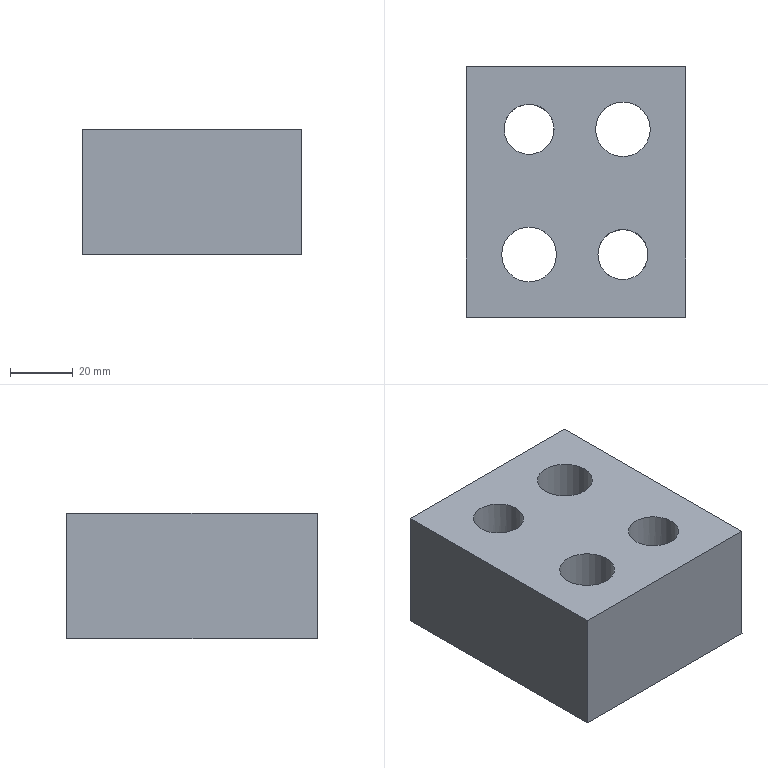Part | NX | features MAIN_BODY 2 | 1 solid | 14 faces | box 70 x 80 x 40 mm | volume 177866 mm3 | plane 8 | cylinder 6 | commonest cylinder face diameters 16 x2 17.5 x2 25.5 x2
STEP:
#1=CARTESIAN_POINT('',(965.,-352.,-70.));
#2=VERTEX_POINT('',#1);
#3=CARTESIAN_POINT('',(965.,-360.,-70.));
#4=DIRECTION('',(0.000000341,0.00000017,-1.));
#5=DIRECTION('',(-0.000000011,1.,0.00000017));
#6=AXIS2_PLACEMENT_3D('',#3,#4,#5);
#7=CIRCLE('',#6,8.);
#8=EDGE_CURVE('',#2,#2,#7,.F.);
#9=ORIENTED_EDGE('',*,*,#8,.T.);
#10=EDGE_LOOP('',(#9));
#11=FACE_BOUND('',#10,.T.);
#12=CARTESIAN_POINT('',(995.,-347.25,-70.));
#13=VERTEX_POINT('',#12);
#14=CARTESIAN_POINT('',(995.,-360.,-70.));
#15=DIRECTION('',(0.000000341,0.00000017,-1.));
#16=DIRECTION('',(-0.000000011,1.,0.00000017));
#17=AXIS2_PLACEMENT_3D('',#14,#15,#16);
#18=CIRCLE('',#17,12.75);
#19=EDGE_CURVE('',#13,#13,#18,.F.);
#20=ORIENTED_EDGE('',*,*,#19,.T.);
#21=EDGE_LOOP('',(#20));
#22=FACE_BOUND('',#21,.T.);
#23=CARTESIAN_POINT('',(945.,-420.,-70.));
#24=VERTEX_POINT('',#23);
#25=CARTESIAN_POINT('',(1015.,-420.,-70.));
#26=VERTEX_POINT('',#25);
#27=CARTESIAN_POINT('',(980.,-420.,-70.));
#28=DIRECTION('',(1.,0.000000011,0.000000341));
#29=VECTOR('',#28,1000.);
#30=LINE('',#27,#29);
#31=EDGE_CURVE('',#24,#26,#30,.T.);
#32=ORIENTED_EDGE('',*,*,#31,.F.);
#33=CARTESIAN_POINT('',(945.,-340.,-70.));
#34=VERTEX_POINT('',#33);
#35=CARTESIAN_POINT('',(945.,-380.,-70.));
#36=DIRECTION('',(0.000000011,-1.,-0.00000017));
#37=VECTOR('',#36,1000.);
#38=LINE('',#35,#37);
#39=EDGE_CURVE('',#34,#24,#38,.T.);
#40=ORIENTED_EDGE('',*,*,#39,.F.);
#41=CARTESIAN_POINT('',(1015.,-340.,-70.));
#42=VERTEX_POINT('',#41);
#43=CARTESIAN_POINT('',(980.,-340.,-70.));
#44=DIRECTION('',(-1.,-0.000000011,-0.000000341));
#45=VECTOR('',#44,1000.);
#46=LINE('',#43,#45);
#47=EDGE_CURVE('',#42,#34,#46,.T.);
#48=ORIENTED_EDGE('',*,*,#47,.F.);
#49=CARTESIAN_POINT('',(1015.,-380.,-70.));
#50=DIRECTION('',(-0.000000011,1.,0.00000017));
#51=VECTOR('',#50,1000.);
#52=LINE('',#49,#51);
#53=EDGE_CURVE('',#26,#42,#52,.T.);
#54=ORIENTED_EDGE('',*,*,#53,.F.);
#55=EDGE_LOOP('',(#32,#40,#48,#54));
#56=FACE_BOUND('',#55,.T.);
#57=CARTESIAN_POINT('',(965.,-387.25,-70.));
#58=VERTEX_POINT('',#57);
#59=CARTESIAN_POINT('',(965.,-400.,-70.));
#60=DIRECTION('',(0.000000341,0.00000017,-1.));
#61=DIRECTION('',(-0.000000011,1.,0.00000017));
#62=AXIS2_PLACEMENT_3D('',#59,#60,#61);
#63=CIRCLE('',#62,12.75);
#64=EDGE_CURVE('',#58,#58,#63,.F.);
#65=ORIENTED_EDGE('',*,*,#64,.T.);
#66=EDGE_LOOP('',(#65));
#67=FACE_BOUND('',#66,.T.);
#68=CARTESIAN_POINT('',(995.,-392.,-70.));
#69=VERTEX_POINT('',#68);
#70=CARTESIAN_POINT('',(995.,-400.,-70.));
#71=DIRECTION('',(0.000000341,0.00000017,-1.));
#72=DIRECTION('',(-0.000000011,1.,0.00000017));
#73=AXIS2_PLACEMENT_3D('',#70,#71,#72);
#74=CIRCLE('',#73,8.);
#75=EDGE_CURVE('',#69,#69,#74,.F.);
#76=ORIENTED_EDGE('',*,*,#75,.T.);
#77=EDGE_LOOP('',(#76));
#78=FACE_BOUND('',#77,.T.);
#79=CARTESIAN_POINT('',(980.,-380.,-70.));
#80=DIRECTION('',(-0.000000341,-0.00000017,1.));
#81=DIRECTION('',(-0.000000011,1.,0.00000017));
#82=AXIS2_PLACEMENT_3D('',#79,#80,#81);
#83=PLANE('',#82);
#84=ADVANCED_FACE('',(#11,#22,#56,#67,#78),#83,.F.);
#85=CARTESIAN_POINT('',(986.25,-360.,-30.));
#86=VERTEX_POINT('',#85);
#87=CARTESIAN_POINT('',(995.,-360.,-30.));
#88=DIRECTION('',(-0.000000341,-0.00000017,1.));
#89=DIRECTION('',(-1.,0.,-0.000000341));
#90=AXIS2_PLACEMENT_3D('',#87,#88,#89);
#91=CIRCLE('',#90,8.75);
#92=EDGE_CURVE('',#86,#86,#91,.F.);
#93=ORIENTED_EDGE('',*,*,#92,.T.);
#94=EDGE_LOOP('',(#93));
#95=FACE_BOUND('',#94,.T.);
#96=CARTESIAN_POINT('',(956.25,-400.,-30.));
#97=VERTEX_POINT('',#96);
#98=CARTESIAN_POINT('',(965.,-400.,-30.));
#99=DIRECTION('',(-0.000000341,-0.00000017,1.));
#100=DIRECTION('',(-1.,0.,-0.000000341));
#101=AXIS2_PLACEMENT_3D('',#98,#99,#100);
#102=CIRCLE('',#101,8.75);
#103=EDGE_CURVE('',#97,#97,#102,.F.);
#104=ORIENTED_EDGE('',*,*,#103,.T.);
#105=EDGE_LOOP('',(#104));
#106=FACE_BOUND('',#105,.T.);
#107=CARTESIAN_POINT('',(957.,-360.,-30.));
#108=VERTEX_POINT('',#107);
#109=CARTESIAN_POINT('',(965.,-360.,-30.));
#110=DIRECTION('',(-0.000000341,-0.00000017,1.));
#111=DIRECTION('',(-1.,0.,-0.000000341));
#112=AXIS2_PLACEMENT_3D('',#109,#110,#111);
#113=CIRCLE('',#112,8.);
#114=EDGE_CURVE('',#108,#108,#113,.T.);
#115=ORIENTED_EDGE('',*,*,#114,.F.);
#116=EDGE_LOOP('',(#115));
#117=FACE_BOUND('',#116,.T.);
#118=CARTESIAN_POINT('',(945.,-420.,-30.));
#119=VERTEX_POINT('',#118);
#120=CARTESIAN_POINT('',(1015.,-420.,-30.));
#121=VERTEX_POINT('',#120);
#122=CARTESIAN_POINT('',(980.,-420.,-30.));
#123=DIRECTION('',(1.,0.000000011,0.000000341));
#124=VECTOR('',#123,1000.);
#125=LINE('',#122,#124);
#126=EDGE_CURVE('',#119,#121,#125,.T.);
#127=ORIENTED_EDGE('',*,*,#126,.T.);
#128=CARTESIAN_POINT('',(1015.,-340.,-30.));
#129=VERTEX_POINT('',#128);
#130=CARTESIAN_POINT('',(1015.,-380.,-30.));
#131=DIRECTION('',(-0.000000011,1.,0.00000017));
#132=VECTOR('',#131,1000.);
#133=LINE('',#130,#132);
#134=EDGE_CURVE('',#121,#129,#133,.T.);
#135=ORIENTED_EDGE('',*,*,#134,.T.);
#136=CARTESIAN_POINT('',(945.,-340.,-30.));
#137=VERTEX_POINT('',#136);
#138=CARTESIAN_POINT('',(980.,-340.,-30.));
#139=DIRECTION('',(-1.,-0.000000011,-0.000000341));
#140=VECTOR('',#139,1000.);
#141=LINE('',#138,#140);
#142=EDGE_CURVE('',#129,#137,#141,.T.);
#143=ORIENTED_EDGE('',*,*,#142,.T.);
#144=CARTESIAN_POINT('',(945.,-380.,-30.));
#145=DIRECTION('',(0.000000011,-1.,-0.00000017));
#146=VECTOR('',#145,1000.);
#147=LINE('',#144,#146);
#148=EDGE_CURVE('',#137,#119,#147,.T.);
#149=ORIENTED_EDGE('',*,*,#148,.T.);
#150=EDGE_LOOP('',(#127,#135,#143,#149));
#151=FACE_BOUND('',#150,.T.);
#152=CARTESIAN_POINT('',(987.,-400.,-30.));
#153=VERTEX_POINT('',#152);
#154=CARTESIAN_POINT('',(995.,-400.,-30.));
#155=DIRECTION('',(-0.000000341,-0.00000017,1.));
#156=DIRECTION('',(-1.,0.,-0.000000341));
#157=AXIS2_PLACEMENT_3D('',#154,#155,#156);
#158=CIRCLE('',#157,8.);
#159=EDGE_CURVE('',#153,#153,#158,.T.);
#160=ORIENTED_EDGE('',*,*,#159,.F.);
#161=EDGE_LOOP('',(#160));
#162=FACE_BOUND('',#161,.T.);
#163=CARTESIAN_POINT('',(980.,-380.,-30.));
#164=DIRECTION('',(-0.000000341,-0.00000017,1.));
#165=DIRECTION('',(-0.000000011,1.,0.00000017));
#166=AXIS2_PLACEMENT_3D('',#163,#164,#165);
#167=PLANE('',#166);
#168=ADVANCED_FACE('',(#95,#106,#117,#151,#162),#167,.T.);
#169=ORIENTED_EDGE('',*,*,#126,.F.);
#170=CARTESIAN_POINT('',(945.,-420.,-70.));
#171=DIRECTION('',(-0.000000341,-0.00000017,1.));
#172=VECTOR('',#171,1000.);
#173=LINE('',#170,#172);
#174=EDGE_CURVE('',#24,#119,#173,.T.);
#175=ORIENTED_EDGE('',*,*,#174,.F.);
#176=ORIENTED_EDGE('',*,*,#31,.T.);
#177=CARTESIAN_POINT('',(1015.,-420.,-70.));
#178=DIRECTION('',(-0.000000341,-0.00000017,1.));
#179=VECTOR('',#178,1000.);
#180=LINE('',#177,#179);
#181=EDGE_CURVE('',#26,#121,#180,.T.);
#182=ORIENTED_EDGE('',*,*,#181,.T.);
#183=EDGE_LOOP('',(#169,#175,#176,#182));
#184=FACE_BOUND('',#183,.T.);
#185=CARTESIAN_POINT('',(980.,-420.,-70.));
#186=DIRECTION('',(-0.000000011,1.,0.00000017));
#187=DIRECTION('',(0.000000341,0.00000017,-1.));
#188=AXIS2_PLACEMENT_3D('',#185,#186,#187);
#189=PLANE('',#188);
#190=ADVANCED_FACE('',(#184),#189,.F.);
#191=ORIENTED_EDGE('',*,*,#148,.F.);
#192=CARTESIAN_POINT('',(945.,-340.,-70.));
#193=DIRECTION('',(-0.000000341,-0.00000017,1.));
#194=VECTOR('',#193,1000.);
#195=LINE('',#192,#194);
#196=EDGE_CURVE('',#34,#137,#195,.T.);
#197=ORIENTED_EDGE('',*,*,#196,.F.);
#198=ORIENTED_EDGE('',*,*,#39,.T.);
#199=ORIENTED_EDGE('',*,*,#174,.T.);
#200=EDGE_LOOP('',(#191,#197,#198,#199));
#201=FACE_BOUND('',#200,.T.);
#202=CARTESIAN_POINT('',(945.,-380.,-70.));
#203=DIRECTION('',(1.,0.000000011,0.000000341));
#204=DIRECTION('',(-0.000000341,-0.00000017,1.));
#205=AXIS2_PLACEMENT_3D('',#202,#203,#204);
#206=PLANE('',#205);
#207=ADVANCED_FACE('',(#201),#206,.F.);
#208=ORIENTED_EDGE('',*,*,#142,.F.);
#209=CARTESIAN_POINT('',(1015.,-340.,-70.));
#210=DIRECTION('',(-0.000000341,-0.00000017,1.));
#211=VECTOR('',#210,1000.);
#212=LINE('',#209,#211);
#213=EDGE_CURVE('',#42,#129,#212,.T.);
#214=ORIENTED_EDGE('',*,*,#213,.F.);
#215=ORIENTED_EDGE('',*,*,#47,.T.);
#216=ORIENTED_EDGE('',*,*,#196,.T.);
#217=EDGE_LOOP('',(#208,#214,#215,#216));
#218=FACE_BOUND('',#217,.T.);
#219=CARTESIAN_POINT('',(980.,-340.,-70.));
#220=DIRECTION('',(0.000000011,-1.,-0.00000017));
#221=DIRECTION('',(-0.000000341,-0.00000017,1.));
#222=AXIS2_PLACEMENT_3D('',#219,#220,#221);
#223=PLANE('',#222);
#224=ADVANCED_FACE('',(#218),#223,.F.);
#225=ORIENTED_EDGE('',*,*,#134,.F.);
#226=ORIENTED_EDGE('',*,*,#181,.F.);
#227=ORIENTED_EDGE('',*,*,#53,.T.);
#228=ORIENTED_EDGE('',*,*,#213,.T.);
#229=EDGE_LOOP('',(#225,#226,#227,#228));
#230=FACE_BOUND('',#229,.T.);
#231=CARTESIAN_POINT('',(1015.,-380.,-70.));
#232=DIRECTION('',(-1.,-0.000000011,-0.000000341));
#233=DIRECTION('',(0.000000341,0.00000017,-1.));
#234=AXIS2_PLACEMENT_3D('',#231,#232,#233);
#235=PLANE('',#234);
#236=ADVANCED_FACE('',(#230),#235,.F.);
#237=CARTESIAN_POINT('',(1007.75,-360.,-50.));
#238=VERTEX_POINT('',#237);
#239=CARTESIAN_POINT('',(995.,-360.,-50.));
#240=DIRECTION('',(0.000000341,0.00000017,-1.));
#241=DIRECTION('',(1.,0.,0.000000341));
#242=AXIS2_PLACEMENT_3D('',#239,#240,#241);
#243=CIRCLE('',#242,12.75);
#244=EDGE_CURVE('',#238,#238,#243,.T.);
#245=ORIENTED_EDGE('',*,*,#244,.F.);
#246=EDGE_LOOP('',(#245));
#247=FACE_BOUND('',#246,.T.);
#248=ORIENTED_EDGE('',*,*,#19,.F.);
#249=EDGE_LOOP('',(#248));
#250=FACE_BOUND('',#249,.T.);
#251=CARTESIAN_POINT('',(995.,-360.,-60.));
#252=DIRECTION('',(0.000000341,0.00000017,-1.));
#253=DIRECTION('',(0.000000011,-1.,-0.00000017));
#254=AXIS2_PLACEMENT_3D('',#251,#252,#253);
#255=CYLINDRICAL_SURFACE('',#254,12.75);
#256=ADVANCED_FACE('',(#247,#250),#255,.F.);
#257=CARTESIAN_POINT('',(1003.75,-360.,-50.));
#258=VERTEX_POINT('',#257);
#259=CARTESIAN_POINT('',(995.,-360.,-50.));
#260=DIRECTION('',(0.000000341,0.00000017,-1.));
#261=DIRECTION('',(1.,0.,0.000000341));
#262=AXIS2_PLACEMENT_3D('',#259,#260,#261);
#263=CIRCLE('',#262,8.75);
#264=EDGE_CURVE('',#258,#258,#263,.F.);
#265=ORIENTED_EDGE('',*,*,#264,.T.);
#266=EDGE_LOOP('',(#265));
#267=FACE_BOUND('',#266,.T.);
#268=ORIENTED_EDGE('',*,*,#244,.T.);
#269=EDGE_LOOP('',(#268));
#270=FACE_BOUND('',#269,.T.);
#271=CARTESIAN_POINT('',(995.,-359.283,-50.));
#272=DIRECTION('',(0.000000341,0.00000017,-1.));
#273=DIRECTION('',(0.000000011,-1.,-0.00000017));
#274=AXIS2_PLACEMENT_3D('',#271,#272,#273);
#275=PLANE('',#274);
#276=ADVANCED_FACE('',(#267,#270),#275,.T.);
#277=CARTESIAN_POINT('',(977.75,-400.,-50.));
#278=VERTEX_POINT('',#277);
#279=CARTESIAN_POINT('',(965.,-400.,-50.));
#280=DIRECTION('',(0.000000341,0.00000017,-1.));
#281=DIRECTION('',(1.,0.,0.000000341));
#282=AXIS2_PLACEMENT_3D('',#279,#280,#281);
#283=CIRCLE('',#282,12.75);
#284=EDGE_CURVE('',#278,#278,#283,.T.);
#285=ORIENTED_EDGE('',*,*,#284,.F.);
#286=EDGE_LOOP('',(#285));
#287=FACE_BOUND('',#286,.T.);
#288=ORIENTED_EDGE('',*,*,#64,.F.);
#289=EDGE_LOOP('',(#288));
#290=FACE_BOUND('',#289,.T.);
#291=CARTESIAN_POINT('',(965.,-400.,-60.));
#292=DIRECTION('',(0.000000341,0.00000017,-1.));
#293=DIRECTION('',(0.000000011,-1.,-0.00000017));
#294=AXIS2_PLACEMENT_3D('',#291,#292,#293);
#295=CYLINDRICAL_SURFACE('',#294,12.75);
#296=ADVANCED_FACE('',(#287,#290),#295,.F.);
#297=CARTESIAN_POINT('',(973.75,-400.,-50.));
#298=VERTEX_POINT('',#297);
#299=CARTESIAN_POINT('',(965.,-400.,-50.));
#300=DIRECTION('',(0.000000341,0.00000017,-1.));
#301=DIRECTION('',(1.,0.,0.000000341));
#302=AXIS2_PLACEMENT_3D('',#299,#300,#301);
#303=CIRCLE('',#302,8.75);
#304=EDGE_CURVE('',#298,#298,#303,.F.);
#305=ORIENTED_EDGE('',*,*,#304,.T.);
#306=EDGE_LOOP('',(#305));
#307=FACE_BOUND('',#306,.T.);
#308=ORIENTED_EDGE('',*,*,#284,.T.);
#309=EDGE_LOOP('',(#308));
#310=FACE_BOUND('',#309,.T.);
#311=CARTESIAN_POINT('',(965.,-399.283,-50.));
#312=DIRECTION('',(0.000000341,0.00000017,-1.));
#313=DIRECTION('',(0.000000011,-1.,-0.00000017));
#314=AXIS2_PLACEMENT_3D('',#311,#312,#313);
#315=PLANE('',#314);
#316=ADVANCED_FACE('',(#307,#310),#315,.T.);
#317=ORIENTED_EDGE('',*,*,#114,.T.);
#318=EDGE_LOOP('',(#317));
#319=FACE_BOUND('',#318,.T.);
#320=ORIENTED_EDGE('',*,*,#8,.F.);
#321=EDGE_LOOP('',(#320));
#322=FACE_BOUND('',#321,.T.);
#323=CARTESIAN_POINT('',(965.,-360.,505.));
#324=DIRECTION('',(0.000000341,0.00000017,-1.));
#325=DIRECTION('',(0.000000011,-1.,-0.00000017));
#326=AXIS2_PLACEMENT_3D('',#323,#324,#325);
#327=CYLINDRICAL_SURFACE('',#326,8.);
#328=ADVANCED_FACE('',(#319,#322),#327,.F.);
#329=ORIENTED_EDGE('',*,*,#159,.T.);
#330=EDGE_LOOP('',(#329));
#331=FACE_BOUND('',#330,.T.);
#332=ORIENTED_EDGE('',*,*,#75,.F.);
#333=EDGE_LOOP('',(#332));
#334=FACE_BOUND('',#333,.T.);
#335=CARTESIAN_POINT('',(995.,-400.,505.));
#336=DIRECTION('',(0.000000341,0.00000017,-1.));
#337=DIRECTION('',(0.000000011,-1.,-0.00000017));
#338=AXIS2_PLACEMENT_3D('',#335,#336,#337);
#339=CYLINDRICAL_SURFACE('',#338,8.);
#340=ADVANCED_FACE('',(#331,#334),#339,.F.);
#341=ORIENTED_EDGE('',*,*,#103,.F.);
#342=EDGE_LOOP('',(#341));
#343=FACE_BOUND('',#342,.T.);
#344=ORIENTED_EDGE('',*,*,#304,.F.);
#345=EDGE_LOOP('',(#344));
#346=FACE_BOUND('',#345,.T.);
#347=CARTESIAN_POINT('',(965.,-400.,-160.));
#348=DIRECTION('',(-0.000000341,-0.00000017,1.));
#349=DIRECTION('',(-1.,0.,-0.000000341));
#350=AXIS2_PLACEMENT_3D('',#347,#348,#349);
#351=CYLINDRICAL_SURFACE('',#350,8.75);
#352=ADVANCED_FACE('',(#343,#346),#351,.F.);
#353=ORIENTED_EDGE('',*,*,#92,.F.);
#354=EDGE_LOOP('',(#353));
#355=FACE_BOUND('',#354,.T.);
#356=ORIENTED_EDGE('',*,*,#264,.F.);
#357=EDGE_LOOP('',(#356));
#358=FACE_BOUND('',#357,.T.);
#359=CARTESIAN_POINT('',(995.,-360.,-160.));
#360=DIRECTION('',(-0.000000341,-0.00000017,1.));
#361=DIRECTION('',(-1.,0.,-0.000000341));
#362=AXIS2_PLACEMENT_3D('',#359,#360,#361);
#363=CYLINDRICAL_SURFACE('',#362,8.75);
#364=ADVANCED_FACE('',(#355,#358),#363,.F.);
#365=CLOSED_SHELL('',(#84,#168,#190,#207,#224,#236,#256,#276,#296,#316,#328,#340,#352,#364));
#366=MANIFOLD_SOLID_BREP('',#365);
#367=(LENGTH_UNIT()NAMED_UNIT(*)SI_UNIT(.MILLI.,.METRE.));
#368=UNCERTAINTY_MEASURE_WITH_UNIT(LENGTH_MEASURE(0.00001),#367,'','');
#369=(NAMED_UNIT(*)PLANE_ANGLE_UNIT()SI_UNIT($,.RADIAN.));
#370=(NAMED_UNIT(*)SI_UNIT($,.STERADIAN.)SOLID_ANGLE_UNIT());
#371=(GEOMETRIC_REPRESENTATION_CONTEXT(3)GLOBAL_UNCERTAINTY_ASSIGNED_CONTEXT((#368))GLOBAL_UNIT_ASSIGNED_CONTEXT((#367,#369,#370))REPRESENTATION_CONTEXT('',''));
#372=ADVANCED_BREP_SHAPE_REPRESENTATION('',(#366),#371);